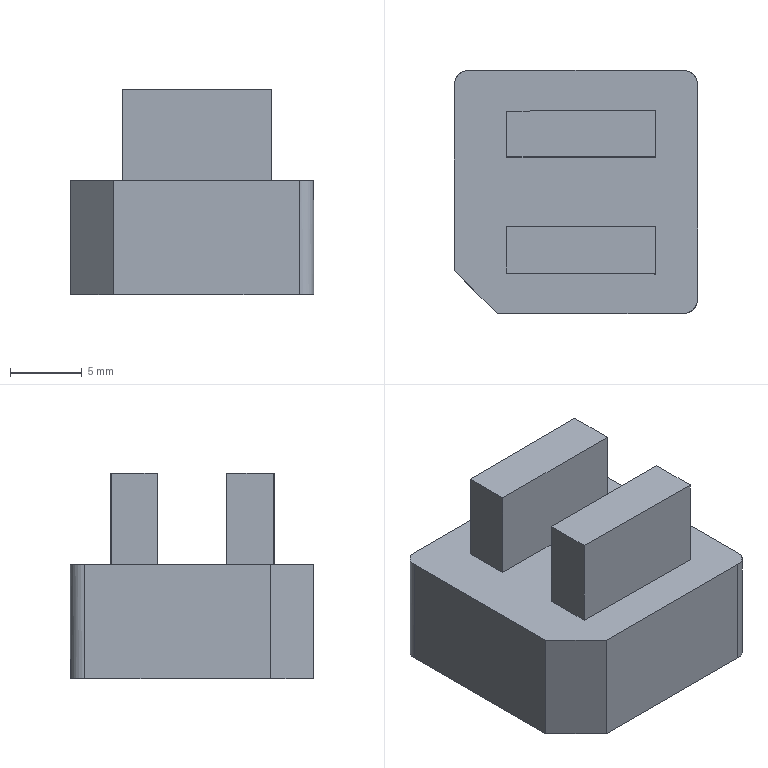NC program | PowerMill | posted with a generic post | part box 17 x 17 x 14.396 mm
Lines 6399 to 6981 of 42940:
N6496 M6
N6497 S8500 M03
N6498 G00 G90 X0.0 Y0.0
N6499 G43 Z11.796 H3
N6500
N6501 G05 P10000 R8
N6502 X16.0359 Y7.373
N6503 Z0.7958
N6504 G01 Z-0.4042 F360.0
N6505 X10.8161 Y6.6124 F600.0
N6506 X-10.0841 Y6.6156
N6507 X-10.1396 Y6.2571
N6508 X-10.1733 Y5.8108
N6509 X-10.1702 Y2.1902
N6510 X10.8912 Y2.187
N6511 X10.8585 Y1.78
N6512 G02 X10.6207 Y0.7307 I-5.5405 J0.7044
N6513 G01 X10.5037 Y0.4135
N6514 X10.3244 Y-0.0201
N6515 X10.5038 Y-0.4135
N6516 X10.6705 Y-0.8878
N6517 X10.7482 Y-1.1733
N6518 G02 X10.8939 Y-2.2384 I-5.3368 J-1.2723
N6519 G01 X-10.221 Y-2.2352
N6520 X-10.2213 Y-5.9107
N6521 X-10.1894 Y-6.3101
N6522 X-10.1344 Y-6.6607
N6523 X10.8158 Y-6.6638
N6524 G00 Z11.796
N6525 G05 P0
N6526 (---------------)
N6527 ( END TOOLPATH : 粗公基准台01-平坦面平行-D10 )
N6528 (---------------)
N6529 ( START TOOLPATH : 粗公基准台01-基准面偏置-D10 )
N6530 (---------------)
N6531 G00 X0.0 Y0.0 Z9.7958
N6532 G05 P10000 R8
N6533 X6.1911 Y19.125
N6534 Z-5.4
N6535 G01 Z-6.6 F360.0
N6536 Y13.85 F600.0
N6537 X0.3931 Y10.9131
N6538 X5.1099 Y10.9377
N6539 X5.8961 Y10.9285
N6540 X6.2891 Y10.8876
N6541 X6.6822 Y10.8164
N6542 X7.0246 Y10.7285
N6543 X7.4684 Y10.5761
N6544 X7.8614 Y10.4027
N6545 X8.2545 Y10.1884
N6546 X8.5159 Y10.0208
N6547 X8.7804 Y9.8268
N6548 X9.0406 Y9.6095
N6549 X9.3374 Y9.3239
N6550 X9.5903 Y9.0406
N6551 X9.8268 Y8.732
N6552 X10.1293 Y8.2545
N6553 X10.3285 Y7.8614
N6554 X10.4878 Y7.4684
N6555 X10.6129 Y7.0722
N6556 X10.7035 Y6.6822
N6557 X10.7641 Y6.2891
N6558 X10.7941 Y5.8961
N6559 X10.7987 Y2.7515
N6560 X10.778 Y1.9654
N6561 X10.7285 Y1.5723
N6562 X10.6475 Y1.1792
N6563 X10.5134 Y0.7228
N6564 X10.3872 Y0.3931
N6565 G03 X10.388 Y-0.3931 I0.9199 J-0.3922
N6566 G01 X10.5134 Y-0.7228
N6567 X10.6475 Y-1.1792
N6568 X10.7285 Y-1.5723
N6569 X10.778 Y-1.9654
N6570 X10.7987 Y-2.7515
N6571 X10.7964 Y-5.8961
N6572 X10.7701 Y-6.2891
N6573 X10.7135 Y-6.6822
N6574 X10.6129 Y-7.1221
N6575 X10.5055 Y-7.4684
N6576 X10.3504 Y-7.8614
N6577 X10.1569 Y-8.2545
N6578 X10.0027 Y-8.5182
N6579 X9.8268 Y-8.7819
N6580 X9.631 Y-9.0406
N6581 X9.3596 Y-9.35
N6582 X9.0406 Y-9.6594
N6583 X8.8433 Y-9.8268
N6584 X8.5489 Y-10.0474
N6585 X8.2545 Y-10.2383
N6586 X7.8753 Y-10.4457
N6587 X7.4684 Y-10.626
N6588 X7.0753 Y-10.7631
N6589 X6.6822 Y-10.8655
N6590 X6.2891 Y-10.9372
N6591 X5.8961 Y-10.9784
N6592 X5.1099 Y-10.9876
N6593 X-5.1099 Y-10.93
N6594 X-5.503 Y-10.8976
N6595 X-5.8961 Y-10.8356
N6596 X-6.2891 Y-10.7414
N6597 X-6.6868 Y-10.6129
N6598 X-7.0776 Y-10.4516
N6599 X-7.4684 Y-10.2506
N6600 X-7.7854 Y-10.0556
N6601 X-8.1025 Y-9.8268
N6602 X-8.2545 Y-9.704
N6603 X-8.6135 Y-9.3723
N6604 X-8.914 Y-9.0406
N6605 X-9.0406 Y-8.8825
N6606 X-9.2636 Y-8.5685
N6607 X-9.4544 Y-8.2545
N6608 X-9.6538 Y-7.8614
N6609 X-9.8268 Y-7.433
N6610 X-9.9438 Y-7.0576
N6611 X-10.031 Y-6.6822
N6612 X-10.0918 Y-6.2891
N6613 X-10.1224 Y-5.8961
N6614 X-10.1259 Y-2.3584
N6615 X-10.1062 Y-1.9654
N6616 X-10.0563 Y-1.5723
N6617 X-9.9757 Y-1.1792
N6618 X-9.8268 Y-0.681
N6619 X-9.7032 Y-0.3669
N6620 G03 X-9.6699 Y0.4049 I-0.9049 J0.4256
N6621 G01 X-9.8268 Y0.8299
N6622 X-9.9258 Y1.1792
N6623 X-10.0059 Y1.5723
N6624 X-10.0563 Y1.9654
N6625 X-10.0763 Y2.7515
N6626 X-10.0702 Y5.8961
N6627 X-10.0356 Y6.2891
N6628 X-9.9711 Y6.6822
N6629 X-9.8268 Y7.235
N6630 X-9.7462 Y7.4684
N6631 X-9.5812 Y7.8614
N6632 X-9.3769 Y8.2545
N6633 X-9.2196 Y8.5105
N6634 X-9.0406 Y8.7666
N6635 X-8.8226 Y9.0406
N6636 X-8.5604 Y9.3262
N6637 X-8.2545 Y9.6118
N6638 X-7.9881 Y9.8268
N6639 X-7.7282 Y10.0109
N6640 X-7.4684 Y10.1723
N6641 X-7.0753 Y10.3796
N6642 X-6.6822 Y10.5469
N6643 X-6.4957 Y10.6129
N6644 X-5.8961 Y10.7757
N6645 X-5.503 Y10.8421
N6646 X-5.1099 Y10.8778
N6647 X-4.3238 Y10.8885
N6648 X0.3931 Y10.9131
N6649 G00 Z9.7958
N6650 G05 P0
N6651 (---------------)
N6652 ( END TOOLPATH : 粗公基准台01-基准面偏置-D10 )
N6653 (---------------)
N6654 ( START TOOLPATH : 粗公基准台01-外形侧光-D10 )
N6655 (---------------)
N6656 G00 X0.0 Y0.0 Z10.796
N6657 G05 P10000 R8
N6658 X10.8676 Y-1.7478
N6659 Z-5.37
N6660 G01 Z-6.57 F360.0
N6661 G03 X10.4281 Y-2.8084 I1.0605 J-1.0609 F600.0
N6662 G01 X10.4276 Y-5.8117
N6663 G02 X8.4691 Y-9.6487 I-4.8795 J0.0723
N6664 G02 X5.5499 Y-10.6194 I-2.921 J3.9093
N6665 G01 X4.1822 Y-10.6123
N6666 X0.3868 Y-10.5924
N6667 X-4.7768 Y-10.5654
N6668 G02 X-9.7547 Y-5.8089 I-0.0945 J4.8841
N6669 G02 X-9.7562 Y-2.4507 I270.8063 J1.8067
N6670 G02 X-9.1432 Y-0.0622 I4.8655 J0.0241
N6671 G03 X-9.1381 Y0.147 I-0.1909 J0.1093
N6672 G02 X-9.7063 Y2.4524 I4.2781 J2.2771
N6673 G01 Y5.5512
N6674 G02 X-4.7762 Y10.5157 I4.8832 J0.0809
N6675 G01 X5.5525 Y10.5696
N6676 G02 X10.4267 Y5.8089 I-0.0043 J-4.88
N6677 G02 X10.4282 Y2.4507 I-294.1914 J-1.8065
N6678 G02 X9.8359 Y0.0997 I-4.875 J-0.022
N6679 G03 Y-0.0994 I0.1962 J-0.0995
N6680 G02 X10.4282 Y-2.4525 I-4.2837 J-2.3293
N6681 G01 X10.4281 Y-2.8084
N6682 G03 X10.8673 Y-3.8692 I1.5 J-0.0003
N6683 G01 X10.7876 Y-1.6932
N6684 G03 X10.3481 Y-2.7538 I1.0605 J-1.0608
N6685 G01 X10.3477 Y-5.8084
N6686 G02 X8.3994 Y-9.6008 I-4.7995 J0.069
N6687 G02 X5.5503 Y-10.5394 I-2.8512 J3.8614
N6688 G01 X4.1826 Y-10.5323
N6689 X0.3872 Y-10.5124
N6690 X-4.7758 Y-10.4854
N6691 G02 X-9.6747 Y-5.8084 I-0.0955 J4.8041
N6692 G02 X-9.6763 Y-2.4524 I270.7117 J1.8071
N6693 G02 X-9.0738 Y-0.102 I4.7854 J0.0258
N6694 G03 X-9.0668 Y0.1833 I-0.2603 J0.1491
N6695 G02 X-9.6263 Y2.4524 I4.2057 J2.2405
N6696 G01 Y5.5503
N6697 G02 X-4.7758 Y10.4357 I4.8031 J0.0818
N6698 G01 X5.5503 Y10.4897
N6699 G02 X10.3467 Y5.8084 I-0.0021 J-4.8
N6700 G02 X10.3482 Y2.4524 I-293.9746 J-1.807
N6701 G02 X9.7646 Y0.1359 I-4.7953 J-0.0237
N6702 G03 Y-0.1356 I0.2675 J-0.1357
N6703 G02 X10.3482 Y-2.4524 I-4.2122 J-2.293
N6704 G01 X10.3481 Y-2.7538
N6705 G03 X10.7873 Y-3.8145 I1.5 J-0.0002
N6706 G00 Z10.796
N6707 G05 P0
N6708 (---------------)
N6709 ( END TOOLPATH : 粗公基准台01-外形侧光-D10 )
N6710 (---------------)
N6711 ( START TOOLPATH : 粗公基准台01-基准台侧光-D10 )
N6712 (---------------)
N6713 G00 X0.0 Y0.0 Z9.7958
N6714 G05 P10000 R8
N6715 X13.8909 Y-16.5452
N6716 Z-13.3
N6717 G01 Z-14.5 F360.0
N6718 G03 X10.9776 Y-12.4816 I-1.4566 J2.0318 F600.0
N6719 G01 X10.8396 Y-12.5806
N6720 X10.8365 Y-12.5827
N6721 X10.8334 Y-12.5846
N6722 X10.3212 Y-12.8853
N6723 X10.318 Y-12.8871
N6724 X10.3149 Y-12.8887
N6725 X9.8679 Y-13.0999
N6726 X9.8649 Y-13.1013
N6727 X9.8618 Y-13.1025
N6728 X9.4148 Y-13.2703
N6729 X9.4118 Y-13.2713
N6730 X9.4087 Y-13.2723
N6731 X8.9617 Y-13.4003
N6732 X8.9591 Y-13.4011
N6733 X8.9564 Y-13.4017
N6734 X8.5527 Y-13.4878
N6735 X8.5495 Y-13.4884
N6736 X8.5463 Y-13.4889
N6737 X8.0561 Y-13.5527
N6738 X8.0532 Y-13.553
N6739 X8.0503 Y-13.5532
N6740 X7.6033 Y-13.5789
N6741 X7.6011 Y-13.579
N6742 X7.5988 Y-13.5791
N6743 X-5.3638 Y-13.58
N6744 X-5.3647
N6745 X-5.3656
N6746 X-5.8125 Y-13.5704
N6747 X-5.816 Y-13.5702
N6748 X-5.8194 Y-13.5699
N6749 X-6.2664 Y-13.5218
N6750 X-6.2689 Y-13.5215
N6751 X-6.2714 Y-13.5211
N6752 X-6.4603 Y-13.4884
N6753 X-6.4621 Y-13.4881
N6754 X-6.4639 Y-13.4877
N6755 X-6.722 Y-13.4308
N6756 X-6.7248 Y-13.4301
N6757 X-6.7277 Y-13.4293
N6758 X-7.1746 Y-13.296
N6759 X-7.1783 Y-13.2948
N6760 X-7.1818 Y-13.2935
N6761 X-7.6288 Y-13.1124
N6762 X-7.6312 Y-13.1114
N6763 X-7.6336 Y-13.1102
N6764 X-7.79 Y-13.0346
N6765 X-7.7918 Y-13.0337
N6766 X-7.7935 Y-13.0328
N6767 X-8.0842 Y-12.8736
N6768 X-8.0871 Y-12.8719
N6769 X-8.09 Y-12.8701
N6770 X-8.5234 Y-12.5822
N6771 X-8.527 Y-12.5797
N6772 X-8.5305 Y-12.5769
N6773 X-8.9912 Y-12.1901
N6774 X-8.9932 Y-12.1883
N6775 X-8.9953 Y-12.1864
N6776 X-9.0577 Y-12.1262
N6777 X-9.0582 Y-12.1257
N6778 X-9.0587 Y-12.1252
N6779 X-12.1252 Y-9.0587
N6780 X-12.1257 Y-9.0582
N6781 X-12.1262 Y-9.0577
N6782 X-12.1864 Y-8.9953
N6783 X-12.1883 Y-8.9933
N6784 X-12.19 Y-8.9913
N6785 X-12.5666 Y-8.5443
N6786 X-12.5694 Y-8.5408
N6787 X-12.572 Y-8.5371
N6788 X-12.87 Y-8.0901
N6789 X-12.8719 Y-8.0872
N6790 X-12.8736 Y-8.0842
N6791 X-13.0328 Y-7.7935
N6792 X-13.0337 Y-7.7918
N6793 X-13.0346 Y-7.79
N6794 X-13.1102 Y-7.6336
N6795 X-13.1114 Y-7.6312
N6796 X-13.1124 Y-7.6288
N6797 X-13.2935 Y-7.1818
N6798 X-13.2948 Y-7.1783
N6799 X-13.296 Y-7.1746
N6800 X-13.4293 Y-6.7277
N6801 X-13.4301 Y-6.7248
N6802 X-13.4308 Y-6.722
N6803 X-13.4877 Y-6.4639
N6804 X-13.4881 Y-6.4621
N6805 X-13.4884 Y-6.4603
N6806 X-13.5211 Y-6.2714
N6807 X-13.5215 Y-6.2689
N6808 X-13.5218 Y-6.2664
N6809 X-13.5699 Y-5.8194
N6810 X-13.5702 Y-5.816
N6811 X-13.5704 Y-5.8125
N6812 X-13.58 Y-5.3656
N6813 Y-5.3647
N6814 Y-5.3638
N6815 X-13.5791 Y7.5988
N6816 X-13.579 Y7.6011
N6817 X-13.5789 Y7.6033
N6818 X-13.5532 Y8.0503
N6819 X-13.553 Y8.053
N6820 X-13.5527 Y8.0557
N6821 X-13.4965 Y8.5027
N6822 X-13.496 Y8.5059
N6823 X-13.4954 Y8.5091
N6824 X-13.4017 Y8.9561
N6825 X-13.4011 Y8.9589
N6826 X-13.4003 Y8.9617
N6827 X-13.2723 Y9.4087
N6828 X-13.2713 Y9.4118
N6829 X-13.2703 Y9.4148
N6830 X-13.1025 Y9.8618
N6831 X-13.1013 Y9.8649
N6832 X-13.0999 Y9.8679
N6833 X-12.8887 Y10.3149
N6834 X-12.8872 Y10.3178
N6835 X-12.8856 Y10.3208
N6836 X-12.6268 Y10.7677
N6837 X-12.6249 Y10.7708
N6838 X-12.6229 Y10.7738
N6839 X-12.3073 Y11.2208
N6840 X-12.3051 Y11.2238
N6841 X-12.3027 Y11.2266
N6842 X-11.9205 Y11.6736
N6843 X-11.9184 Y11.676
N6844 X-11.9163 Y11.6782
N6845 X-11.6782 Y11.9163
N6846 X-11.676 Y11.9184
N6847 X-11.6736 Y11.9205
N6848 X-11.2266 Y12.3027
N6849 X-11.224 Y12.3049
N6850 X-11.2213 Y12.307
N6851 X-10.8396 Y12.5806
N6852 X-10.8365 Y12.5827
N6853 X-10.8334 Y12.5846
N6854 X-10.3212 Y12.8853
N6855 X-10.318 Y12.8871
N6856 X-10.3149 Y12.8887
N6857 X-9.8679 Y13.0999
N6858 X-9.8649 Y13.1013
N6859 X-9.8618 Y13.1025
N6860 X-9.4148 Y13.2703
N6861 X-9.4118 Y13.2713
N6862 X-9.4087 Y13.2723
N6863 X-8.9617 Y13.4003
N6864 X-8.9591 Y13.4011
N6865 X-8.9564 Y13.4017
N6866 X-8.5527 Y13.4878
N6867 X-8.5495 Y13.4884
N6868 X-8.5463 Y13.4889
N6869 X-8.0561 Y13.5527
N6870 X-8.0532 Y13.553
N6871 X-8.0503 Y13.5532
N6872 X-7.6033 Y13.5789
N6873 X-7.6011 Y13.579
N6874 X-7.5988 Y13.5791
N6875 X0.0
N6876 X7.5988
N6877 X7.6011 Y13.579
N6878 X7.6033 Y13.5789
N6879 X8.0503 Y13.5532
N6880 X8.053 Y13.553
N6881 X8.0557 Y13.5527
N6882 X8.5027 Y13.4965
N6883 X8.5059 Y13.496
N6884 X8.5091 Y13.4954
N6885 X8.9561 Y13.4017
N6886 X8.9589 Y13.4011
N6887 X8.9617 Y13.4003
N6888 X9.4087 Y13.2723
N6889 X9.4118 Y13.2713
N6890 X9.4148 Y13.2703
N6891 X9.8618 Y13.1025
N6892 X9.8649 Y13.1013
N6893 X9.8679 Y13.0999
N6894 X10.3149 Y12.8887
N6895 X10.3178 Y12.8872
N6896 X10.3208 Y12.8856
N6897 X10.7677 Y12.6268
N6898 X10.7708 Y12.6249
N6899 X10.7738 Y12.6229
N6900 X11.2208 Y12.3073
N6901 X11.2238 Y12.3051
N6902 X11.2266 Y12.3027
N6903 X11.6736 Y11.9205
N6904 X11.676 Y11.9184
N6905 X11.6782 Y11.9163
N6906 X11.9163 Y11.6782
N6907 X11.9184 Y11.676
N6908 X11.9205 Y11.6736
N6909 X12.3027 Y11.2266
N6910 X12.3049 Y11.224
N6911 X12.307 Y11.2213
N6912 X12.5806 Y10.8396
N6913 X12.5827 Y10.8365
N6914 X12.5846 Y10.8334
N6915 X12.8853 Y10.3212
N6916 X12.8871 Y10.318
N6917 X12.8887 Y10.3149
N6918 X13.0999 Y9.8679
N6919 X13.1013 Y9.8649
N6920 X13.1025 Y9.8618
N6921 X13.2703 Y9.4148
N6922 X13.2713 Y9.4118
N6923 X13.2723 Y9.4087
N6924 X13.4003 Y8.9617
N6925 X13.4011 Y8.9591
N6926 X13.4017 Y8.9564
N6927 X13.4878 Y8.5527
N6928 X13.4884 Y8.5495
N6929 X13.4889 Y8.5463
N6930 X13.5527 Y8.0561
N6931 X13.553 Y8.0532
N6932 X13.5532 Y8.0503
N6933 X13.5789 Y7.6033
N6934 X13.579 Y7.6011
N6935 X13.5791 Y7.5988
N6936 Y-7.5988
N6937 X13.579 Y-7.6011
N6938 X13.5789 Y-7.6033
N6939 X13.5532 Y-8.0503
N6940 X13.553 Y-8.053
N6941 X13.5527 Y-8.0557
N6942 X13.4965 Y-8.5027
N6943 X13.496 Y-8.5059
N6944 X13.4954 Y-8.5091
N6945 X13.4017 Y-8.9561
N6946 X13.4011 Y-8.9589
N6947 X13.4003 Y-8.9617
N6948 X13.2723 Y-9.4087
N6949 X13.2713 Y-9.4118
N6950 X13.2703 Y-9.4148
N6951 X13.1025 Y-9.8618
N6952 X13.1013 Y-9.8649
N6953 X13.0999 Y-9.8679
N6954 X12.8887 Y-10.3149
N6955 X12.8872 Y-10.3178
N6956 X12.8856 Y-10.3208
N6957 X12.6268 Y-10.7677
N6958 X12.6249 Y-10.7708
N6959 X12.6229 Y-10.7738
N6960 X12.3073 Y-11.2208
N6961 X12.3051 Y-11.2238
N6962 X12.3027 Y-11.2266
N6963 X11.9205 Y-11.6736
N6964 X11.9184 Y-11.676
N6965 X11.9163 Y-11.6782
N6966 X11.6782 Y-11.9163
N6967 X11.676 Y-11.9184
N6968 X11.6736 Y-11.9205
N6969 X11.2266 Y-12.3027
N6970 X11.224 Y-12.3049
N6971 X11.2213 Y-12.307
N6972 X10.9776 Y-12.4816
N6973 G03 X13.8909 Y-16.5452 I1.4567 J-2.0318
N6974 G01 X13.8395 Y-16.4836
N6975 G03 X10.9262 Y-12.42 I-1.4566 J2.0318
N6976 G01 X10.7929 Y-12.5156
N6977 X10.2807 Y-12.8163
N6978 X9.8337 Y-13.0276
N6979 X9.3867 Y-13.1954
N6980 X8.9397 Y-13.3234
N6981 X8.536 Y-13.4096
N6982 X8.0457 Y-13.4734
N6983 X7.5988 Y-13.4991
N6984 X-5.3638 Y-13.5
N6985 X-5.8108 Y-13.4904
N6986 X-6.2578 Y-13.4422
N6987 X-6.4467 Y-13.4096
N6988 X-6.7048 Y-13.3527
N6989 X-7.1518 Y-13.2193
N6990 X-7.5988 Y-13.0382
N6991 X-7.7551 Y-12.9626
N6992 X-8.0457 Y-12.8034
N6993 X-8.4791 Y-12.5156
N6994 X-8.9397 Y-12.1289
N6995 X-9.0022 Y-12.0686
N6996 X-12.0686 Y-9.0022
N6997 X-12.1289 Y-8.9397
N6998 X-12.5055 Y-8.4927
N6999 X-12.8034 Y-8.0457
N7000 X-12.9626 Y-7.7551
N7001 X-13.0382 Y-7.5988
N7002 X-13.2193 Y-7.1518
N7003 X-13.3527 Y-6.7048
N7004 X-13.4096 Y-6.4467
N7005 X-13.4422 Y-6.2578
N7006 X-13.4904 Y-5.8108
N7007 X-13.5 Y-5.3638
N7008 X-13.4991 Y7.5988
N7009 X-13.4734 Y8.0457
N7010 X-13.4171 Y8.4927
N7011 X-13.3234 Y8.9397
N7012 X-13.1954 Y9.3867
N7013 X-13.0276 Y9.8337
N7014 X-12.8163 Y10.2807
N7015 X-12.5576 Y10.7277
N7016 X-12.2419 Y11.1746
N7017 X-11.8597 Y11.6216
N7018 X-11.6216 Y11.8597
N7019 X-11.1746 Y12.2419
N7020 X-10.7929 Y12.5156
N7021 X-10.2807 Y12.8163
N7022 X-9.8337 Y13.0276
N7023 X-9.3867 Y13.1954
N7024 X-8.9397 Y13.3234
N7025 X-8.536 Y13.4096
N7026 X-8.0457 Y13.4734
N7027 X-7.5988 Y13.4991
N7028 X0.0
N7029 X7.5988
N7030 X8.0457 Y13.4734
N7031 X8.4927 Y13.4171
N7032 X8.9397 Y13.3234
N7033 X9.3867 Y13.1954
N7034 X9.8337 Y13.0276
N7035 X10.2807 Y12.8163
N7036 X10.7277 Y12.5576
N7037 X11.1746 Y12.2419
N7038 X11.6216 Y11.8597
N7039 X11.8597 Y11.6216
N7040 X12.2419 Y11.1746
N7041 X12.5156 Y10.7929
N7042 X12.8163 Y10.2807
N7043 X13.0276 Y9.8337
N7044 X13.1954 Y9.3867
N7045 X13.3234 Y8.9397
N7046 X13.4096 Y8.536
N7047 X13.4734 Y8.0457
N7048 X13.4991 Y7.5988
N7049 Y-7.5988
N7050 X13.4734 Y-8.0457
N7051 X13.4171 Y-8.4927
N7052 X13.3234 Y-8.9397
N7053 X13.1954 Y-9.3867
N7054 X13.0276 Y-9.8337
N7055 X12.8163 Y-10.2807
N7056 X12.5576 Y-10.7277
N7057 X12.2419 Y-11.1746
N7058 X11.8597 Y-11.6216
N7059 X11.6216 Y-11.8597
N7060 X11.1746 Y-12.2419
N7061 X10.9262 Y-12.42
N7062 G03 X13.8395 Y-16.4836 I1.4567 J-2.0318
N7063 G00 Z9.7958
N7064 G05 P0
N7065 (---------------)
N7066 ( END TOOLPATH : 粗公基准台01-基准台侧光-D10 )
N7067 (---------------)
N7068
N7069 M05
N7070 G53 Z0.0
N7071 (---------------)
N7072 ( START TOOLPATH : 粗公精光01-等高-D3 )
N7073 (---------------)
N7074 ( TOOL NO.    :10 )
N7075 ( TOOL TYPE   : ENDMILL)
N7076 ( TOOL ID     : D3_3)
N7077 ( TOOL DIA    : 3.0 LENGTH 61.44)
N7078 T10